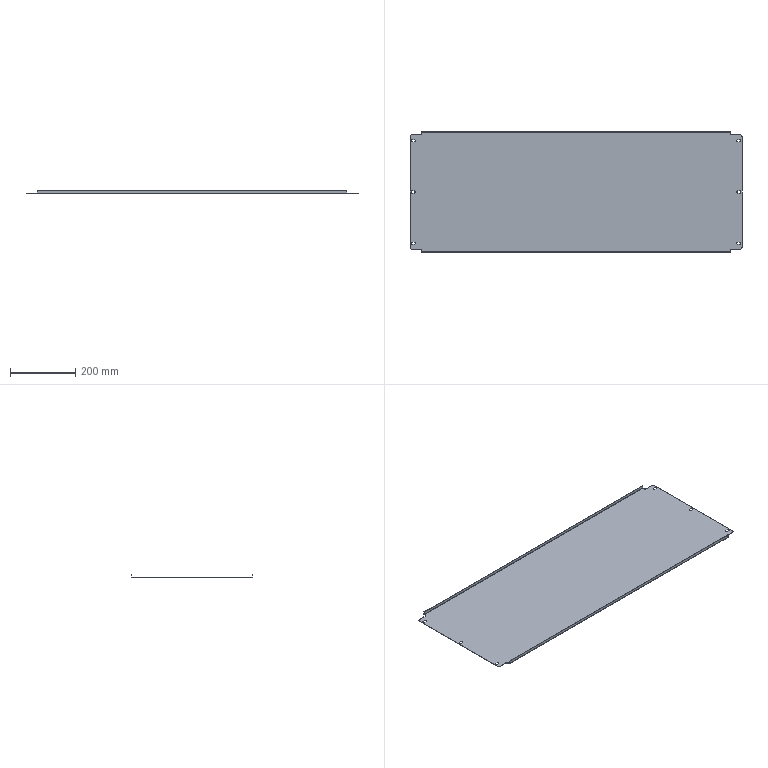Part | SolidWorks | features ICE 3, Cut 1, EdgeFlange 1, Fillet 1, FlatPattern 1, SMBaseFlange 1, SheetMetal 1 | 1 solid | 68 faces | box 1020 x 371 x 10 mm | volume 392822 mm3 | plane 38 | cylinder 30 | commonest cylinder face diameters 7 x18 10 x8 1 x2 3 x2